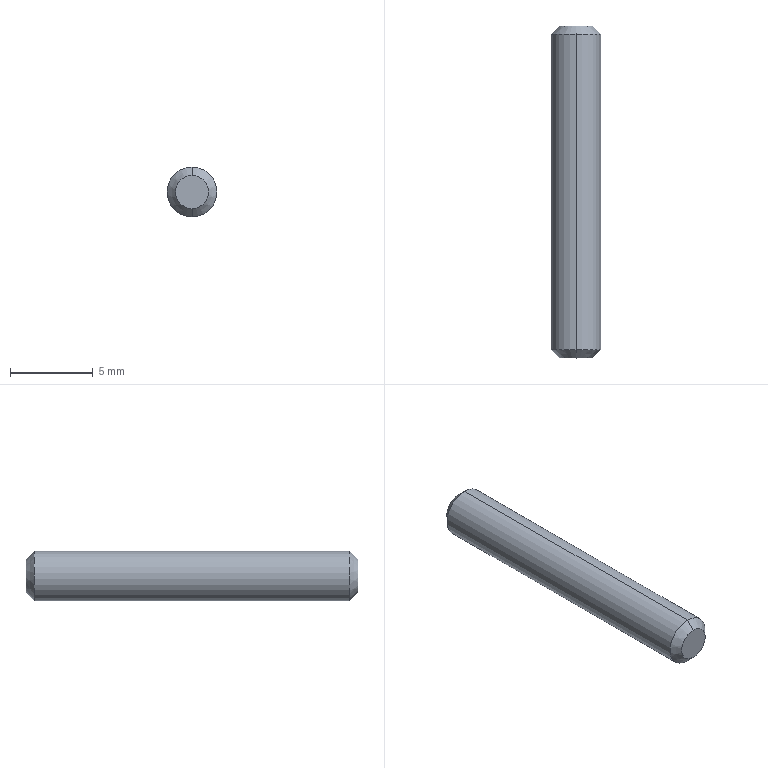Part | NX | features BREP 1 | 1 solid | 8 faces | box 3 x 20 x 3 mm | volume 139.277 mm3 | cone 4 | cylinder 2 | plane 2 | commonest cylinder face diameters 3 x2
STEP:
#1=CARTESIAN_POINT('',(0.,20.,1.));
#2=VERTEX_POINT('',#1);
#3=CARTESIAN_POINT('',(0.,20.,-1.));
#4=VERTEX_POINT('',#3);
#5=CARTESIAN_POINT('',(0.,20.,0.));
#6=DIRECTION('',(0.,1.,0.));
#7=DIRECTION('',(0.,0.,1.));
#8=AXIS2_PLACEMENT_3D('',#5,#6,#7);
#9=CIRCLE('',#8,1.);
#10=EDGE_CURVE('',#2,#4,#9,.T.);
#11=ORIENTED_EDGE('',*,*,#10,.F.);
#12=CARTESIAN_POINT('',(0.,19.5,1.5));
#13=VERTEX_POINT('',#12);
#14=CARTESIAN_POINT('',(0.,20.,1.));
#15=DIRECTION('',(0.,-0.7071,0.7071));
#16=VECTOR('',#15,1000.);
#17=LINE('',#14,#16);
#18=EDGE_CURVE('',#2,#13,#17,.T.);
#19=ORIENTED_EDGE('',*,*,#18,.T.);
#20=CARTESIAN_POINT('',(0.,19.5,-1.5));
#21=VERTEX_POINT('',#20);
#22=CARTESIAN_POINT('',(0.,19.5,0.));
#23=DIRECTION('',(0.,-1.,0.));
#24=DIRECTION('',(0.,0.,1.));
#25=AXIS2_PLACEMENT_3D('',#22,#23,#24);
#26=CIRCLE('',#25,1.5);
#27=EDGE_CURVE('',#21,#13,#26,.T.);
#28=ORIENTED_EDGE('',*,*,#27,.F.);
#29=CARTESIAN_POINT('',(0.,20.,-1.));
#30=DIRECTION('',(0.,-0.7071,-0.7071));
#31=VECTOR('',#30,1000.);
#32=LINE('',#29,#31);
#33=EDGE_CURVE('',#4,#21,#32,.T.);
#34=ORIENTED_EDGE('',*,*,#33,.F.);
#35=EDGE_LOOP('',(#11,#19,#28,#34));
#36=FACE_BOUND('',#35,.T.);
#37=CARTESIAN_POINT('',(0.,20.,0.));
#38=DIRECTION('',(0.,-1.,0.));
#39=DIRECTION('',(0.,0.,-1.));
#40=AXIS2_PLACEMENT_3D('',#37,#38,#39);
#41=CONICAL_SURFACE('',#40,1.,0.7854);
#42=ADVANCED_FACE('',(#36),#41,.T.);
#43=CARTESIAN_POINT('',(0.,0.,-1.));
#44=VERTEX_POINT('',#43);
#45=CARTESIAN_POINT('',(0.,0.,1.));
#46=VERTEX_POINT('',#45);
#47=CARTESIAN_POINT('',(0.,0.,0.));
#48=DIRECTION('',(0.,-1.,0.));
#49=DIRECTION('',(0.,0.,1.));
#50=AXIS2_PLACEMENT_3D('',#47,#48,#49);
#51=CIRCLE('',#50,1.);
#52=EDGE_CURVE('',#44,#46,#51,.T.);
#53=ORIENTED_EDGE('',*,*,#52,.F.);
#54=CARTESIAN_POINT('',(0.,0.5,-1.5));
#55=VERTEX_POINT('',#54);
#56=CARTESIAN_POINT('',(0.,0.5,-1.5));
#57=DIRECTION('',(0.,0.7071,-0.7071));
#58=VECTOR('',#57,1000.);
#59=LINE('',#56,#58);
#60=EDGE_CURVE('',#55,#44,#59,.F.);
#61=ORIENTED_EDGE('',*,*,#60,.F.);
#62=CARTESIAN_POINT('',(0.,0.5,1.5));
#63=VERTEX_POINT('',#62);
#64=CARTESIAN_POINT('',(0.,0.5,0.));
#65=DIRECTION('',(0.,1.,0.));
#66=DIRECTION('',(0.,0.,1.));
#67=AXIS2_PLACEMENT_3D('',#64,#65,#66);
#68=CIRCLE('',#67,1.5);
#69=EDGE_CURVE('',#63,#55,#68,.T.);
#70=ORIENTED_EDGE('',*,*,#69,.F.);
#71=CARTESIAN_POINT('',(0.,0.5,1.5));
#72=DIRECTION('',(0.,0.7071,0.7071));
#73=VECTOR('',#72,1000.);
#74=LINE('',#71,#73);
#75=EDGE_CURVE('',#63,#46,#74,.F.);
#76=ORIENTED_EDGE('',*,*,#75,.T.);
#77=EDGE_LOOP('',(#53,#61,#70,#76));
#78=FACE_BOUND('',#77,.T.);
#79=CARTESIAN_POINT('',(0.,0.5,0.));
#80=DIRECTION('',(0.,1.,0.));
#81=DIRECTION('',(0.,0.,1.));
#82=AXIS2_PLACEMENT_3D('',#79,#80,#81);
#83=CONICAL_SURFACE('',#82,1.5,0.7854);
#84=ADVANCED_FACE('',(#78),#83,.T.);
#85=ORIENTED_EDGE('',*,*,#27,.T.);
#86=CARTESIAN_POINT('',(0.,20.,1.5));
#87=DIRECTION('',(0.,-1.,0.));
#88=VECTOR('',#87,1000.);
#89=LINE('',#86,#88);
#90=EDGE_CURVE('',#13,#63,#89,.T.);
#91=ORIENTED_EDGE('',*,*,#90,.T.);
#92=ORIENTED_EDGE('',*,*,#69,.T.);
#93=CARTESIAN_POINT('',(0.,20.,-1.5));
#94=DIRECTION('',(0.,-1.,0.));
#95=VECTOR('',#94,1000.);
#96=LINE('',#93,#95);
#97=EDGE_CURVE('',#21,#55,#96,.T.);
#98=ORIENTED_EDGE('',*,*,#97,.F.);
#99=EDGE_LOOP('',(#85,#91,#92,#98));
#100=FACE_BOUND('',#99,.T.);
#101=CARTESIAN_POINT('',(0.,20.,0.));
#102=DIRECTION('',(0.,-1.,0.));
#103=DIRECTION('',(0.,0.,-1.));
#104=AXIS2_PLACEMENT_3D('',#101,#102,#103);
#105=CYLINDRICAL_SURFACE('',#104,1.5);
#106=ADVANCED_FACE('',(#100),#105,.T.);
#107=ORIENTED_EDGE('',*,*,#90,.F.);
#108=CARTESIAN_POINT('',(0.,19.5,0.));
#109=DIRECTION('',(0.,-1.,0.));
#110=DIRECTION('',(0.,0.,1.));
#111=AXIS2_PLACEMENT_3D('',#108,#109,#110);
#112=CIRCLE('',#111,1.5);
#113=EDGE_CURVE('',#13,#21,#112,.T.);
#114=ORIENTED_EDGE('',*,*,#113,.T.);
#115=ORIENTED_EDGE('',*,*,#97,.T.);
#116=CARTESIAN_POINT('',(0.,0.5,0.));
#117=DIRECTION('',(0.,1.,0.));
#118=DIRECTION('',(0.,0.,1.));
#119=AXIS2_PLACEMENT_3D('',#116,#117,#118);
#120=CIRCLE('',#119,1.5);
#121=EDGE_CURVE('',#55,#63,#120,.T.);
#122=ORIENTED_EDGE('',*,*,#121,.T.);
#123=EDGE_LOOP('',(#107,#114,#115,#122));
#124=FACE_BOUND('',#123,.T.);
#125=CARTESIAN_POINT('',(0.,20.,0.));
#126=DIRECTION('',(0.,-1.,0.));
#127=DIRECTION('',(0.,0.,-1.));
#128=AXIS2_PLACEMENT_3D('',#125,#126,#127);
#129=CYLINDRICAL_SURFACE('',#128,1.5);
#130=ADVANCED_FACE('',(#124),#129,.T.);
#131=CARTESIAN_POINT('',(0.,20.,0.));
#132=DIRECTION('',(0.,1.,0.));
#133=DIRECTION('',(0.,0.,1.));
#134=AXIS2_PLACEMENT_3D('',#131,#132,#133);
#135=CIRCLE('',#134,1.);
#136=EDGE_CURVE('',#4,#2,#135,.T.);
#137=ORIENTED_EDGE('',*,*,#136,.T.);
#138=ORIENTED_EDGE('',*,*,#10,.T.);
#139=EDGE_LOOP('',(#137,#138));
#140=FACE_BOUND('',#139,.T.);
#141=CARTESIAN_POINT('',(0.,20.,0.));
#142=DIRECTION('',(0.,1.,0.));
#143=DIRECTION('',(1.,0.,0.));
#144=AXIS2_PLACEMENT_3D('',#141,#142,#143);
#145=PLANE('',#144);
#146=ADVANCED_FACE('',(#140),#145,.T.);
#147=CARTESIAN_POINT('',(0.,0.,0.));
#148=DIRECTION('',(0.,-1.,0.));
#149=DIRECTION('',(0.,0.,1.));
#150=AXIS2_PLACEMENT_3D('',#147,#148,#149);
#151=CIRCLE('',#150,1.);
#152=EDGE_CURVE('',#46,#44,#151,.T.);
#153=ORIENTED_EDGE('',*,*,#152,.T.);
#154=ORIENTED_EDGE('',*,*,#52,.T.);
#155=EDGE_LOOP('',(#153,#154));
#156=FACE_BOUND('',#155,.T.);
#157=CARTESIAN_POINT('',(0.,0.,0.));
#158=DIRECTION('',(0.,1.,0.));
#159=DIRECTION('',(1.,0.,0.));
#160=AXIS2_PLACEMENT_3D('',#157,#158,#159);
#161=PLANE('',#160);
#162=ADVANCED_FACE('',(#156),#161,.F.);
#163=ORIENTED_EDGE('',*,*,#60,.T.);
#164=ORIENTED_EDGE('',*,*,#152,.F.);
#165=ORIENTED_EDGE('',*,*,#75,.F.);
#166=ORIENTED_EDGE('',*,*,#121,.F.);
#167=EDGE_LOOP('',(#163,#164,#165,#166));
#168=FACE_BOUND('',#167,.T.);
#169=CARTESIAN_POINT('',(0.,0.5,0.));
#170=DIRECTION('',(0.,1.,0.));
#171=DIRECTION('',(0.,0.,1.));
#172=AXIS2_PLACEMENT_3D('',#169,#170,#171);
#173=CONICAL_SURFACE('',#172,1.5,0.7854);
#174=ADVANCED_FACE('',(#168),#173,.T.);
#175=ORIENTED_EDGE('',*,*,#18,.F.);
#176=ORIENTED_EDGE('',*,*,#136,.F.);
#177=ORIENTED_EDGE('',*,*,#33,.T.);
#178=ORIENTED_EDGE('',*,*,#113,.F.);
#179=EDGE_LOOP('',(#175,#176,#177,#178));
#180=FACE_BOUND('',#179,.T.);
#181=CARTESIAN_POINT('',(0.,20.,0.));
#182=DIRECTION('',(0.,-1.,0.));
#183=DIRECTION('',(0.,0.,-1.));
#184=AXIS2_PLACEMENT_3D('',#181,#182,#183);
#185=CONICAL_SURFACE('',#184,1.,0.7854);
#186=ADVANCED_FACE('',(#180),#185,.T.);
#187=CLOSED_SHELL('',(#42,#84,#106,#130,#146,#162,#174,#186));
#188=MANIFOLD_SOLID_BREP('',#187);
#189=(LENGTH_UNIT()NAMED_UNIT(*)SI_UNIT(.MILLI.,.METRE.));
#190=UNCERTAINTY_MEASURE_WITH_UNIT(LENGTH_MEASURE(0.00001),#189,'','');
#191=(NAMED_UNIT(*)PLANE_ANGLE_UNIT()SI_UNIT($,.RADIAN.));
#192=(NAMED_UNIT(*)SI_UNIT($,.STERADIAN.)SOLID_ANGLE_UNIT());
#193=(GEOMETRIC_REPRESENTATION_CONTEXT(3)GLOBAL_UNCERTAINTY_ASSIGNED_CONTEXT((#190))GLOBAL_UNIT_ASSIGNED_CONTEXT((#189,#191,#192))REPRESENTATION_CONTEXT('',''));
#194=ADVANCED_BREP_SHAPE_REPRESENTATION('',(#188),#193);